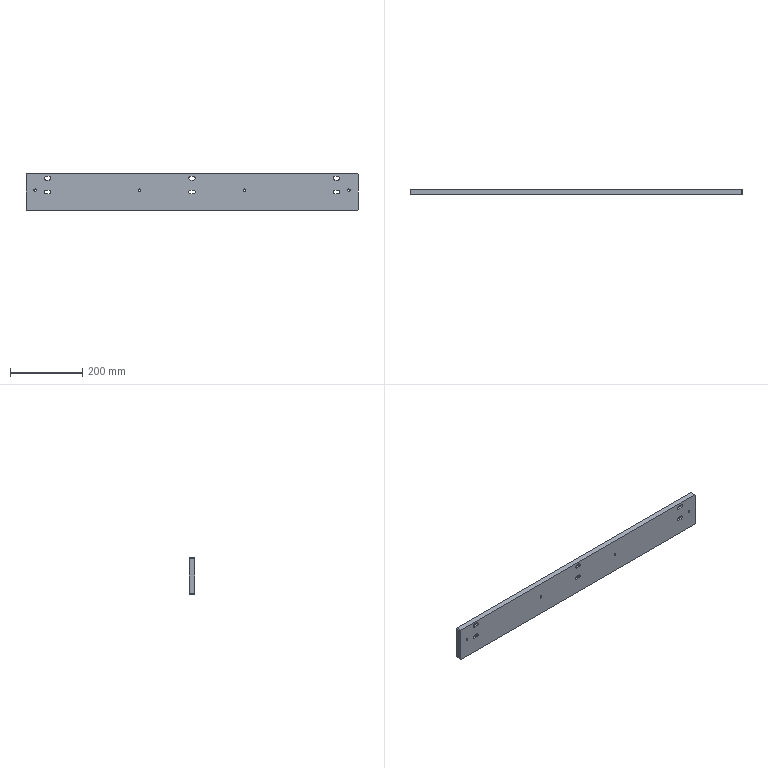Part | NX | features BREP 1 | 1 solid | 72 faces | box 920 x 15 x 100 mm | volume 1355971 mm3 | plane 40 | cylinder 32 | commonest cylinder face diameters 10 x12 15 x12 6.8 x8